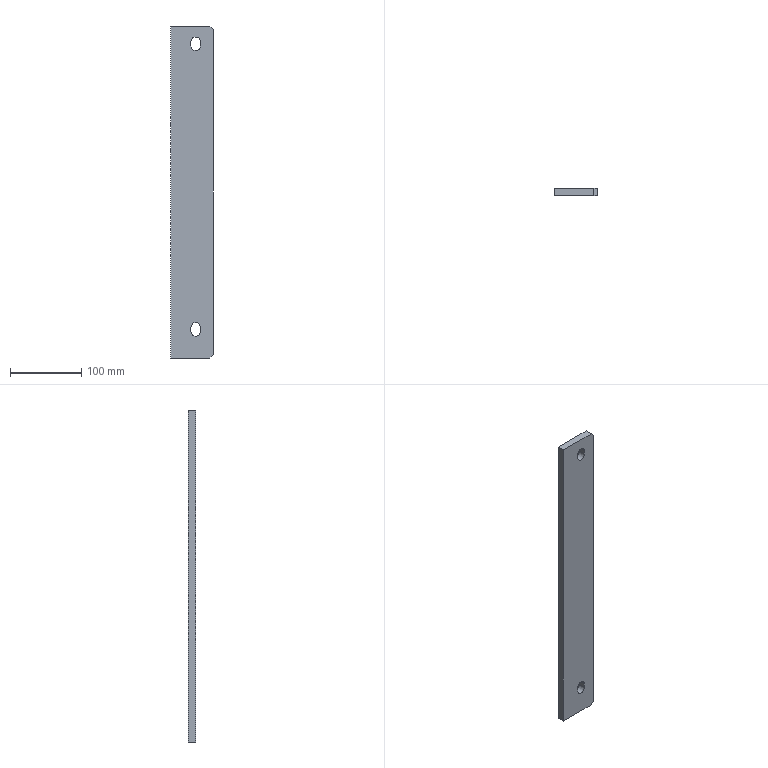Part | NX | features solid 2 | 1 solid | 16 faces | box 60 x 10 x 465 mm | volume 274535 mm3 | plane 12 | cylinder 4 | commonest cylinder face diameters 13 x4
STEP:
#1=CARTESIAN_POINT('',(1060.,0.,-55.));
#2=VERTEX_POINT('',#1);
#3=CARTESIAN_POINT('',(1055.,0.,-50.));
#4=VERTEX_POINT('',#3);
#5=CARTESIAN_POINT('',(1055.,0.,-50.));
#6=DIRECTION('',(-0.7071,0.,0.7071));
#7=VECTOR('',#6,1000.);
#8=LINE('',#5,#7);
#9=EDGE_CURVE('',#2,#4,#8,.T.);
#10=ORIENTED_EDGE('',*,*,#9,.F.);
#11=CARTESIAN_POINT('',(1060.,10.,-55.));
#12=VERTEX_POINT('',#11);
#13=CARTESIAN_POINT('',(1060.,0.,-55.));
#14=DIRECTION('',(0.,-1.,0.));
#15=VECTOR('',#14,1000.);
#16=LINE('',#13,#15);
#17=EDGE_CURVE('',#12,#2,#16,.T.);
#18=ORIENTED_EDGE('',*,*,#17,.F.);
#19=CARTESIAN_POINT('',(1055.,10.,-50.));
#20=VERTEX_POINT('',#19);
#21=CARTESIAN_POINT('',(1290.,10.,-285.));
#22=DIRECTION('',(0.7071,0.,-0.7071));
#23=VECTOR('',#22,1000.);
#24=LINE('',#21,#23);
#25=EDGE_CURVE('',#20,#12,#24,.T.);
#26=ORIENTED_EDGE('',*,*,#25,.F.);
#27=CARTESIAN_POINT('',(1055.,10.,-50.));
#28=DIRECTION('',(0.,1.,0.));
#29=VECTOR('',#28,1000.);
#30=LINE('',#27,#29);
#31=EDGE_CURVE('',#4,#20,#30,.T.);
#32=ORIENTED_EDGE('',*,*,#31,.F.);
#33=EDGE_LOOP('',(#10,#18,#26,#32));
#34=FACE_BOUND('',#33,.T.);
#35=CARTESIAN_POINT('',(1055.,10.,-50.));
#36=DIRECTION('',(-0.7071,0.,-0.7071));
#37=DIRECTION('',(-0.7071,0.,0.7071));
#38=AXIS2_PLACEMENT_3D('',#35,#36,#37);
#39=PLANE('',#38);
#40=ADVANCED_FACE('',(#34),#39,.F.);
#41=CARTESIAN_POINT('',(1060.,10.,-510.));
#42=VERTEX_POINT('',#41);
#43=CARTESIAN_POINT('',(1055.,10.,-515.));
#44=VERTEX_POINT('',#43);
#45=CARTESIAN_POINT('',(1057.5,10.,-512.5));
#46=DIRECTION('',(-0.7071,0.,-0.7071));
#47=VECTOR('',#46,1000.);
#48=LINE('',#45,#47);
#49=EDGE_CURVE('',#42,#44,#48,.T.);
#50=ORIENTED_EDGE('',*,*,#49,.F.);
#51=CARTESIAN_POINT('',(1060.,0.,-510.));
#52=VERTEX_POINT('',#51);
#53=CARTESIAN_POINT('',(1060.,0.,-510.));
#54=DIRECTION('',(0.,1.,0.));
#55=VECTOR('',#54,1000.);
#56=LINE('',#53,#55);
#57=EDGE_CURVE('',#52,#42,#56,.T.);
#58=ORIENTED_EDGE('',*,*,#57,.F.);
#59=CARTESIAN_POINT('',(1055.,0.,-515.));
#60=VERTEX_POINT('',#59);
#61=CARTESIAN_POINT('',(1055.,0.,-515.));
#62=DIRECTION('',(0.7071,0.,0.7071));
#63=VECTOR('',#62,1000.);
#64=LINE('',#61,#63);
#65=EDGE_CURVE('',#60,#52,#64,.T.);
#66=ORIENTED_EDGE('',*,*,#65,.F.);
#67=CARTESIAN_POINT('',(1055.,0.,-515.));
#68=DIRECTION('',(0.,-1.,0.));
#69=VECTOR('',#68,1000.);
#70=LINE('',#67,#69);
#71=EDGE_CURVE('',#44,#60,#70,.T.);
#72=ORIENTED_EDGE('',*,*,#71,.F.);
#73=EDGE_LOOP('',(#50,#58,#66,#72));
#74=FACE_BOUND('',#73,.T.);
#75=CARTESIAN_POINT('',(1055.,0.,-515.));
#76=DIRECTION('',(-0.7071,0.,0.7071));
#77=DIRECTION('',(0.,1.,0.));
#78=AXIS2_PLACEMENT_3D('',#75,#76,#77);
#79=PLANE('',#78);
#80=ADVANCED_FACE('',(#74),#79,.F.);
#81=CARTESIAN_POINT('',(1041.5,0.,-472.));
#82=VERTEX_POINT('',#81);
#83=CARTESIAN_POINT('',(1041.5,10.,-472.));
#84=VERTEX_POINT('',#83);
#85=CARTESIAN_POINT('',(1041.5,-458.962,-472.));
#86=DIRECTION('',(0.,1.,0.));
#87=VECTOR('',#86,1000.);
#88=LINE('',#85,#87);
#89=EDGE_CURVE('',#82,#84,#88,.T.);
#90=ORIENTED_EDGE('',*,*,#89,.T.);
#91=CARTESIAN_POINT('',(1041.5,10.,-478.));
#92=VERTEX_POINT('',#91);
#93=CARTESIAN_POINT('',(1041.5,10.,-472.));
#94=DIRECTION('',(0.,0.,-1.));
#95=VECTOR('',#94,1000.);
#96=LINE('',#93,#95);
#97=EDGE_CURVE('',#84,#92,#96,.T.);
#98=ORIENTED_EDGE('',*,*,#97,.T.);
#99=CARTESIAN_POINT('',(1041.5,0.,-478.));
#100=VERTEX_POINT('',#99);
#101=CARTESIAN_POINT('',(1041.5,-458.962,-478.));
#102=DIRECTION('',(0.,1.,0.));
#103=VECTOR('',#102,1000.);
#104=LINE('',#101,#103);
#105=EDGE_CURVE('',#100,#92,#104,.T.);
#106=ORIENTED_EDGE('',*,*,#105,.F.);
#107=CARTESIAN_POINT('',(1041.5,0.,-515.));
#108=DIRECTION('',(0.,0.,-1.));
#109=VECTOR('',#108,1000.);
#110=LINE('',#107,#109);
#111=EDGE_CURVE('',#82,#100,#110,.T.);
#112=ORIENTED_EDGE('',*,*,#111,.F.);
#113=EDGE_LOOP('',(#90,#98,#106,#112));
#114=FACE_BOUND('',#113,.T.);
#115=CARTESIAN_POINT('',(1041.5,-458.962,-472.));
#116=DIRECTION('',(1.,0.,0.));
#117=DIRECTION('',(0.,-1.,0.));
#118=AXIS2_PLACEMENT_3D('',#115,#116,#117);
#119=PLANE('',#118);
#120=ADVANCED_FACE('',(#114),#119,.F.);
#121=CARTESIAN_POINT('',(1028.5,0.,-472.));
#122=VERTEX_POINT('',#121);
#123=CARTESIAN_POINT('',(1028.5,10.,-472.));
#124=VERTEX_POINT('',#123);
#125=CARTESIAN_POINT('',(1028.5,-458.962,-472.));
#126=DIRECTION('',(0.,1.,0.));
#127=VECTOR('',#126,1000.);
#128=LINE('',#125,#127);
#129=EDGE_CURVE('',#122,#124,#128,.T.);
#130=ORIENTED_EDGE('',*,*,#129,.T.);
#131=CARTESIAN_POINT('',(1035.,10.,-472.));
#132=DIRECTION('',(0.,1.,0.));
#133=DIRECTION('',(0.,0.,-1.));
#134=AXIS2_PLACEMENT_3D('',#131,#132,#133);
#135=CIRCLE('',#134,6.5);
#136=EDGE_CURVE('',#124,#84,#135,.T.);
#137=ORIENTED_EDGE('',*,*,#136,.T.);
#138=ORIENTED_EDGE('',*,*,#89,.F.);
#139=CARTESIAN_POINT('',(1035.,0.,-472.));
#140=DIRECTION('',(0.,1.,0.));
#141=DIRECTION('',(-1.,0.,0.));
#142=AXIS2_PLACEMENT_3D('',#139,#140,#141);
#143=CIRCLE('',#142,6.5);
#144=EDGE_CURVE('',#122,#82,#143,.T.);
#145=ORIENTED_EDGE('',*,*,#144,.F.);
#146=EDGE_LOOP('',(#130,#137,#138,#145));
#147=FACE_BOUND('',#146,.T.);
#148=CARTESIAN_POINT('',(1035.,-458.962,-472.));
#149=DIRECTION('',(0.,1.,0.));
#150=DIRECTION('',(-1.,0.,0.));
#151=AXIS2_PLACEMENT_3D('',#148,#149,#150);
#152=CYLINDRICAL_SURFACE('',#151,6.5);
#153=ADVANCED_FACE('',(#147),#152,.F.);
#154=CARTESIAN_POINT('',(1028.5,0.,-478.));
#155=VERTEX_POINT('',#154);
#156=CARTESIAN_POINT('',(1028.5,10.,-478.));
#157=VERTEX_POINT('',#156);
#158=CARTESIAN_POINT('',(1028.5,-458.962,-478.));
#159=DIRECTION('',(0.,1.,0.));
#160=VECTOR('',#159,1000.);
#161=LINE('',#158,#160);
#162=EDGE_CURVE('',#155,#157,#161,.T.);
#163=ORIENTED_EDGE('',*,*,#162,.T.);
#164=CARTESIAN_POINT('',(1028.5,10.,-472.));
#165=DIRECTION('',(0.,0.,1.));
#166=VECTOR('',#165,1000.);
#167=LINE('',#164,#166);
#168=EDGE_CURVE('',#157,#124,#167,.T.);
#169=ORIENTED_EDGE('',*,*,#168,.T.);
#170=ORIENTED_EDGE('',*,*,#129,.F.);
#171=CARTESIAN_POINT('',(1028.5,0.,-515.));
#172=DIRECTION('',(0.,0.,1.));
#173=VECTOR('',#172,1000.);
#174=LINE('',#171,#173);
#175=EDGE_CURVE('',#155,#122,#174,.T.);
#176=ORIENTED_EDGE('',*,*,#175,.F.);
#177=EDGE_LOOP('',(#163,#169,#170,#176));
#178=FACE_BOUND('',#177,.T.);
#179=CARTESIAN_POINT('',(1028.5,-458.962,-472.));
#180=DIRECTION('',(-1.,0.,0.));
#181=DIRECTION('',(0.,0.,1.));
#182=AXIS2_PLACEMENT_3D('',#179,#180,#181);
#183=PLANE('',#182);
#184=ADVANCED_FACE('',(#178),#183,.F.);
#185=ORIENTED_EDGE('',*,*,#105,.T.);
#186=CARTESIAN_POINT('',(1035.,10.,-478.));
#187=DIRECTION('',(0.,1.,0.));
#188=DIRECTION('',(0.,0.,1.));
#189=AXIS2_PLACEMENT_3D('',#186,#187,#188);
#190=CIRCLE('',#189,6.5);
#191=EDGE_CURVE('',#92,#157,#190,.T.);
#192=ORIENTED_EDGE('',*,*,#191,.T.);
#193=ORIENTED_EDGE('',*,*,#162,.F.);
#194=CARTESIAN_POINT('',(1035.,0.,-478.));
#195=DIRECTION('',(0.,1.,0.));
#196=DIRECTION('',(-1.,0.,0.));
#197=AXIS2_PLACEMENT_3D('',#194,#195,#196);
#198=CIRCLE('',#197,6.5);
#199=EDGE_CURVE('',#100,#155,#198,.T.);
#200=ORIENTED_EDGE('',*,*,#199,.F.);
#201=EDGE_LOOP('',(#185,#192,#193,#200));
#202=FACE_BOUND('',#201,.T.);
#203=CARTESIAN_POINT('',(1035.,-458.962,-478.));
#204=DIRECTION('',(0.,1.,0.));
#205=DIRECTION('',(-1.,0.,0.));
#206=AXIS2_PLACEMENT_3D('',#203,#204,#205);
#207=CYLINDRICAL_SURFACE('',#206,6.5);
#208=ADVANCED_FACE('',(#202),#207,.F.);
#209=CARTESIAN_POINT('',(1041.5,0.,-72.));
#210=VERTEX_POINT('',#209);
#211=CARTESIAN_POINT('',(1041.5,10.,-72.));
#212=VERTEX_POINT('',#211);
#213=CARTESIAN_POINT('',(1041.5,-458.962,-72.));
#214=DIRECTION('',(0.,1.,0.));
#215=VECTOR('',#214,1000.);
#216=LINE('',#213,#215);
#217=EDGE_CURVE('',#210,#212,#216,.T.);
#218=ORIENTED_EDGE('',*,*,#217,.T.);
#219=CARTESIAN_POINT('',(1041.5,10.,-78.));
#220=VERTEX_POINT('',#219);
#221=CARTESIAN_POINT('',(1041.5,10.,-72.));
#222=DIRECTION('',(0.,0.,-1.));
#223=VECTOR('',#222,1000.);
#224=LINE('',#221,#223);
#225=EDGE_CURVE('',#212,#220,#224,.T.);
#226=ORIENTED_EDGE('',*,*,#225,.T.);
#227=CARTESIAN_POINT('',(1041.5,0.,-78.));
#228=VERTEX_POINT('',#227);
#229=CARTESIAN_POINT('',(1041.5,-458.962,-78.));
#230=DIRECTION('',(0.,1.,0.));
#231=VECTOR('',#230,1000.);
#232=LINE('',#229,#231);
#233=EDGE_CURVE('',#228,#220,#232,.T.);
#234=ORIENTED_EDGE('',*,*,#233,.F.);
#235=CARTESIAN_POINT('',(1041.5,0.,-515.));
#236=DIRECTION('',(0.,0.,-1.));
#237=VECTOR('',#236,1000.);
#238=LINE('',#235,#237);
#239=EDGE_CURVE('',#210,#228,#238,.T.);
#240=ORIENTED_EDGE('',*,*,#239,.F.);
#241=EDGE_LOOP('',(#218,#226,#234,#240));
#242=FACE_BOUND('',#241,.T.);
#243=CARTESIAN_POINT('',(1041.5,-458.962,-72.));
#244=DIRECTION('',(1.,0.,0.));
#245=DIRECTION('',(0.,-1.,0.));
#246=AXIS2_PLACEMENT_3D('',#243,#244,#245);
#247=PLANE('',#246);
#248=ADVANCED_FACE('',(#242),#247,.F.);
#249=CARTESIAN_POINT('',(1028.5,0.,-72.));
#250=VERTEX_POINT('',#249);
#251=CARTESIAN_POINT('',(1028.5,10.,-72.));
#252=VERTEX_POINT('',#251);
#253=CARTESIAN_POINT('',(1028.5,-458.962,-72.));
#254=DIRECTION('',(0.,1.,0.));
#255=VECTOR('',#254,1000.);
#256=LINE('',#253,#255);
#257=EDGE_CURVE('',#250,#252,#256,.T.);
#258=ORIENTED_EDGE('',*,*,#257,.T.);
#259=CARTESIAN_POINT('',(1035.,10.,-72.));
#260=DIRECTION('',(0.,1.,0.));
#261=DIRECTION('',(0.,0.,-1.));
#262=AXIS2_PLACEMENT_3D('',#259,#260,#261);
#263=CIRCLE('',#262,6.5);
#264=EDGE_CURVE('',#252,#212,#263,.T.);
#265=ORIENTED_EDGE('',*,*,#264,.T.);
#266=ORIENTED_EDGE('',*,*,#217,.F.);
#267=CARTESIAN_POINT('',(1035.,0.,-72.));
#268=DIRECTION('',(0.,1.,0.));
#269=DIRECTION('',(-1.,0.,0.));
#270=AXIS2_PLACEMENT_3D('',#267,#268,#269);
#271=CIRCLE('',#270,6.5);
#272=EDGE_CURVE('',#250,#210,#271,.T.);
#273=ORIENTED_EDGE('',*,*,#272,.F.);
#274=EDGE_LOOP('',(#258,#265,#266,#273));
#275=FACE_BOUND('',#274,.T.);
#276=CARTESIAN_POINT('',(1035.,-458.962,-72.));
#277=DIRECTION('',(0.,1.,0.));
#278=DIRECTION('',(-1.,0.,0.));
#279=AXIS2_PLACEMENT_3D('',#276,#277,#278);
#280=CYLINDRICAL_SURFACE('',#279,6.5);
#281=ADVANCED_FACE('',(#275),#280,.F.);
#282=CARTESIAN_POINT('',(1028.5,0.,-78.));
#283=VERTEX_POINT('',#282);
#284=CARTESIAN_POINT('',(1028.5,10.,-78.));
#285=VERTEX_POINT('',#284);
#286=CARTESIAN_POINT('',(1028.5,-458.962,-78.));
#287=DIRECTION('',(0.,1.,0.));
#288=VECTOR('',#287,1000.);
#289=LINE('',#286,#288);
#290=EDGE_CURVE('',#283,#285,#289,.T.);
#291=ORIENTED_EDGE('',*,*,#290,.T.);
#292=CARTESIAN_POINT('',(1028.5,10.,-72.));
#293=DIRECTION('',(0.,0.,1.));
#294=VECTOR('',#293,1000.);
#295=LINE('',#292,#294);
#296=EDGE_CURVE('',#285,#252,#295,.T.);
#297=ORIENTED_EDGE('',*,*,#296,.T.);
#298=ORIENTED_EDGE('',*,*,#257,.F.);
#299=CARTESIAN_POINT('',(1028.5,0.,-515.));
#300=DIRECTION('',(0.,0.,1.));
#301=VECTOR('',#300,1000.);
#302=LINE('',#299,#301);
#303=EDGE_CURVE('',#283,#250,#302,.T.);
#304=ORIENTED_EDGE('',*,*,#303,.F.);
#305=EDGE_LOOP('',(#291,#297,#298,#304));
#306=FACE_BOUND('',#305,.T.);
#307=CARTESIAN_POINT('',(1028.5,-458.962,-72.));
#308=DIRECTION('',(-1.,0.,0.));
#309=DIRECTION('',(0.,0.,1.));
#310=AXIS2_PLACEMENT_3D('',#307,#308,#309);
#311=PLANE('',#310);
#312=ADVANCED_FACE('',(#306),#311,.F.);
#313=ORIENTED_EDGE('',*,*,#233,.T.);
#314=CARTESIAN_POINT('',(1035.,10.,-78.));
#315=DIRECTION('',(0.,1.,0.));
#316=DIRECTION('',(0.,0.,1.));
#317=AXIS2_PLACEMENT_3D('',#314,#315,#316);
#318=CIRCLE('',#317,6.5);
#319=EDGE_CURVE('',#220,#285,#318,.T.);
#320=ORIENTED_EDGE('',*,*,#319,.T.);
#321=ORIENTED_EDGE('',*,*,#290,.F.);
#322=CARTESIAN_POINT('',(1035.,0.,-78.));
#323=DIRECTION('',(0.,1.,0.));
#324=DIRECTION('',(-1.,0.,0.));
#325=AXIS2_PLACEMENT_3D('',#322,#323,#324);
#326=CIRCLE('',#325,6.5);
#327=EDGE_CURVE('',#228,#283,#326,.T.);
#328=ORIENTED_EDGE('',*,*,#327,.F.);
#329=EDGE_LOOP('',(#313,#320,#321,#328));
#330=FACE_BOUND('',#329,.T.);
#331=CARTESIAN_POINT('',(1035.,-458.962,-78.));
#332=DIRECTION('',(0.,1.,0.));
#333=DIRECTION('',(-1.,0.,0.));
#334=AXIS2_PLACEMENT_3D('',#331,#332,#333);
#335=CYLINDRICAL_SURFACE('',#334,6.5);
#336=ADVANCED_FACE('',(#330),#335,.F.);
#337=CARTESIAN_POINT('',(1000.,0.,-50.));
#338=VERTEX_POINT('',#337);
#339=CARTESIAN_POINT('',(1000.,10.,-50.));
#340=VERTEX_POINT('',#339);
#341=CARTESIAN_POINT('',(1000.,0.,-50.));
#342=DIRECTION('',(0.,1.,0.));
#343=VECTOR('',#342,1000.);
#344=LINE('',#341,#343);
#345=EDGE_CURVE('',#338,#340,#344,.T.);
#346=ORIENTED_EDGE('',*,*,#345,.T.);
#347=CARTESIAN_POINT('',(1000.,10.,-515.));
#348=VERTEX_POINT('',#347);
#349=CARTESIAN_POINT('',(1000.,10.,-50.));
#350=DIRECTION('',(0.,0.,1.));
#351=VECTOR('',#350,1000.);
#352=LINE('',#349,#351);
#353=EDGE_CURVE('',#348,#340,#352,.T.);
#354=ORIENTED_EDGE('',*,*,#353,.F.);
#355=CARTESIAN_POINT('',(1000.,0.,-515.));
#356=VERTEX_POINT('',#355);
#357=CARTESIAN_POINT('',(1000.,0.,-515.));
#358=DIRECTION('',(0.,-1.,0.));
#359=VECTOR('',#358,1000.);
#360=LINE('',#357,#359);
#361=EDGE_CURVE('',#348,#356,#360,.T.);
#362=ORIENTED_EDGE('',*,*,#361,.T.);
#363=CARTESIAN_POINT('',(1000.,0.,-50.));
#364=DIRECTION('',(0.,0.,1.));
#365=VECTOR('',#364,1000.);
#366=LINE('',#363,#365);
#367=EDGE_CURVE('',#356,#338,#366,.T.);
#368=ORIENTED_EDGE('',*,*,#367,.T.);
#369=EDGE_LOOP('',(#346,#354,#362,#368));
#370=FACE_BOUND('',#369,.T.);
#371=CARTESIAN_POINT('',(1000.,0.,-50.));
#372=DIRECTION('',(1.,0.,0.));
#373=DIRECTION('',(0.,-1.,0.));
#374=AXIS2_PLACEMENT_3D('',#371,#372,#373);
#375=PLANE('',#374);
#376=ADVANCED_FACE('',(#370),#375,.F.);
#377=CARTESIAN_POINT('',(1060.,0.,-50.));
#378=DIRECTION('',(1.,0.,0.));
#379=VECTOR('',#378,1000.);
#380=LINE('',#377,#379);
#381=EDGE_CURVE('',#338,#4,#380,.T.);
#382=ORIENTED_EDGE('',*,*,#381,.T.);
#383=ORIENTED_EDGE('',*,*,#31,.T.);
#384=CARTESIAN_POINT('',(1060.,10.,-50.));
#385=DIRECTION('',(1.,0.,0.));
#386=VECTOR('',#385,1000.);
#387=LINE('',#384,#386);
#388=EDGE_CURVE('',#340,#20,#387,.T.);
#389=ORIENTED_EDGE('',*,*,#388,.F.);
#390=ORIENTED_EDGE('',*,*,#345,.F.);
#391=EDGE_LOOP('',(#382,#383,#389,#390));
#392=FACE_BOUND('',#391,.T.);
#393=CARTESIAN_POINT('',(1060.,10.,-50.));
#394=DIRECTION('',(0.,0.,-1.));
#395=DIRECTION('',(-1.,0.,0.));
#396=AXIS2_PLACEMENT_3D('',#393,#394,#395);
#397=PLANE('',#396);
#398=ADVANCED_FACE('',(#392),#397,.F.);
#399=ORIENTED_EDGE('',*,*,#319,.F.);
#400=ORIENTED_EDGE('',*,*,#225,.F.);
#401=ORIENTED_EDGE('',*,*,#264,.F.);
#402=ORIENTED_EDGE('',*,*,#296,.F.);
#403=EDGE_LOOP('',(#399,#400,#401,#402));
#404=FACE_BOUND('',#403,.T.);
#405=ORIENTED_EDGE('',*,*,#191,.F.);
#406=ORIENTED_EDGE('',*,*,#97,.F.);
#407=ORIENTED_EDGE('',*,*,#136,.F.);
#408=ORIENTED_EDGE('',*,*,#168,.F.);
#409=EDGE_LOOP('',(#405,#406,#407,#408));
#410=FACE_BOUND('',#409,.T.);
#411=CARTESIAN_POINT('',(1060.,10.,-515.));
#412=DIRECTION('',(0.,0.,-1.));
#413=VECTOR('',#412,1000.);
#414=LINE('',#411,#413);
#415=EDGE_CURVE('',#12,#42,#414,.T.);
#416=ORIENTED_EDGE('',*,*,#415,.T.);
#417=ORIENTED_EDGE('',*,*,#49,.T.);
#418=CARTESIAN_POINT('',(1060.,10.,-515.));
#419=DIRECTION('',(-1.,0.,0.));
#420=VECTOR('',#419,1000.);
#421=LINE('',#418,#420);
#422=EDGE_CURVE('',#44,#348,#421,.T.);
#423=ORIENTED_EDGE('',*,*,#422,.T.);
#424=ORIENTED_EDGE('',*,*,#353,.T.);
#425=ORIENTED_EDGE('',*,*,#388,.T.);
#426=ORIENTED_EDGE('',*,*,#25,.T.);
#427=EDGE_LOOP('',(#416,#417,#423,#424,#425,#426));
#428=FACE_BOUND('',#427,.T.);
#429=CARTESIAN_POINT('',(1060.,10.,-515.));
#430=DIRECTION('',(0.,1.,0.));
#431=DIRECTION('',(1.,0.,0.));
#432=AXIS2_PLACEMENT_3D('',#429,#430,#431);
#433=PLANE('',#432);
#434=ADVANCED_FACE('',(#404,#410,#428),#433,.T.);
#435=ORIENTED_EDGE('',*,*,#422,.F.);
#436=ORIENTED_EDGE('',*,*,#71,.T.);
#437=CARTESIAN_POINT('',(1060.,0.,-515.));
#438=DIRECTION('',(-1.,0.,0.));
#439=VECTOR('',#438,1000.);
#440=LINE('',#437,#439);
#441=EDGE_CURVE('',#60,#356,#440,.T.);
#442=ORIENTED_EDGE('',*,*,#441,.T.);
#443=ORIENTED_EDGE('',*,*,#361,.F.);
#444=EDGE_LOOP('',(#435,#436,#442,#443));
#445=FACE_BOUND('',#444,.T.);
#446=CARTESIAN_POINT('',(1060.,0.,-515.));
#447=DIRECTION('',(0.,0.,1.));
#448=DIRECTION('',(0.,-1.,0.));
#449=AXIS2_PLACEMENT_3D('',#446,#447,#448);
#450=PLANE('',#449);
#451=ADVANCED_FACE('',(#445),#450,.F.);
#452=ORIENTED_EDGE('',*,*,#239,.T.);
#453=ORIENTED_EDGE('',*,*,#327,.T.);
#454=ORIENTED_EDGE('',*,*,#303,.T.);
#455=ORIENTED_EDGE('',*,*,#272,.T.);
#456=EDGE_LOOP('',(#452,#453,#454,#455));
#457=FACE_BOUND('',#456,.T.);
#458=ORIENTED_EDGE('',*,*,#111,.T.);
#459=ORIENTED_EDGE('',*,*,#199,.T.);
#460=ORIENTED_EDGE('',*,*,#175,.T.);
#461=ORIENTED_EDGE('',*,*,#144,.T.);
#462=EDGE_LOOP('',(#458,#459,#460,#461));
#463=FACE_BOUND('',#462,.T.);
#464=ORIENTED_EDGE('',*,*,#441,.F.);
#465=ORIENTED_EDGE('',*,*,#65,.T.);
#466=CARTESIAN_POINT('',(1060.,0.,-515.));
#467=DIRECTION('',(0.,0.,1.));
#468=VECTOR('',#467,1000.);
#469=LINE('',#466,#468);
#470=EDGE_CURVE('',#52,#2,#469,.T.);
#471=ORIENTED_EDGE('',*,*,#470,.T.);
#472=ORIENTED_EDGE('',*,*,#9,.T.);
#473=ORIENTED_EDGE('',*,*,#381,.F.);
#474=ORIENTED_EDGE('',*,*,#367,.F.);
#475=EDGE_LOOP('',(#464,#465,#471,#472,#473,#474));
#476=FACE_BOUND('',#475,.T.);
#477=CARTESIAN_POINT('',(1060.,0.,-515.));
#478=DIRECTION('',(0.,1.,0.));
#479=DIRECTION('',(1.,0.,0.));
#480=AXIS2_PLACEMENT_3D('',#477,#478,#479);
#481=PLANE('',#480);
#482=ADVANCED_FACE('',(#457,#463,#476),#481,.F.);
#483=ORIENTED_EDGE('',*,*,#470,.F.);
#484=ORIENTED_EDGE('',*,*,#57,.T.);
#485=ORIENTED_EDGE('',*,*,#415,.F.);
#486=ORIENTED_EDGE('',*,*,#17,.T.);
#487=EDGE_LOOP('',(#483,#484,#485,#486));
#488=FACE_BOUND('',#487,.T.);
#489=CARTESIAN_POINT('',(1060.,0.,-515.));
#490=DIRECTION('',(-1.,0.,0.));
#491=DIRECTION('',(0.,0.,1.));
#492=AXIS2_PLACEMENT_3D('',#489,#490,#491);
#493=PLANE('',#492);
#494=ADVANCED_FACE('',(#488),#493,.F.);
#495=CLOSED_SHELL('',(#40,#80,#120,#153,#184,#208,#248,#281,#312,#336,#376,#398,#434,#451,#482,#494));
#496=MANIFOLD_SOLID_BREP('',#495);
#497=(LENGTH_UNIT()NAMED_UNIT(*)SI_UNIT(.MILLI.,.METRE.));
#498=UNCERTAINTY_MEASURE_WITH_UNIT(LENGTH_MEASURE(0.00001),#497,'','');
#499=(NAMED_UNIT(*)PLANE_ANGLE_UNIT()SI_UNIT($,.RADIAN.));
#500=(NAMED_UNIT(*)SI_UNIT($,.STERADIAN.)SOLID_ANGLE_UNIT());
#501=(GEOMETRIC_REPRESENTATION_CONTEXT(3)GLOBAL_UNCERTAINTY_ASSIGNED_CONTEXT((#498))GLOBAL_UNIT_ASSIGNED_CONTEXT((#497,#499,#500))REPRESENTATION_CONTEXT('',''));
#502=ADVANCED_BREP_SHAPE_REPRESENTATION('',(#496),#501);